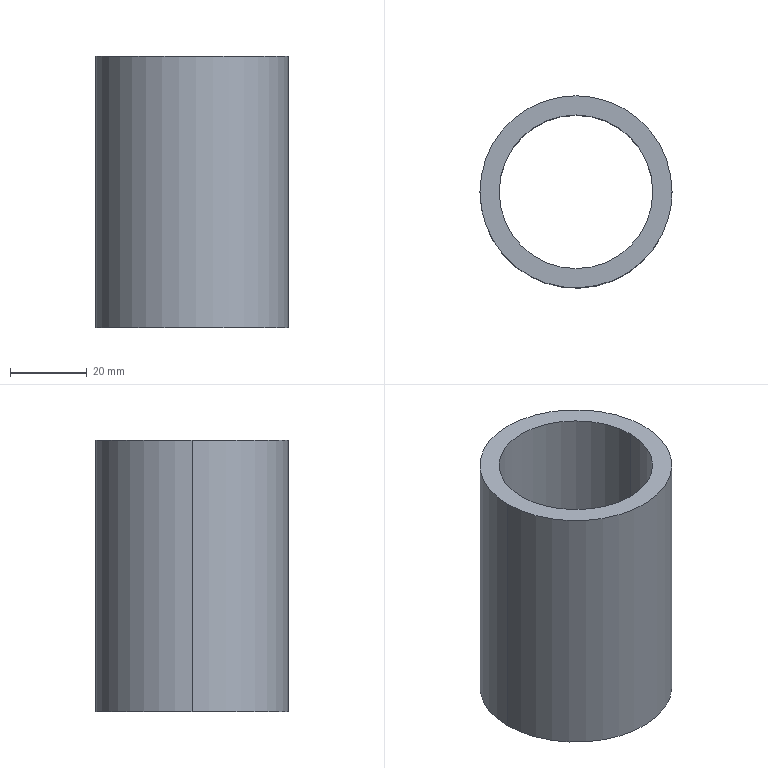Part | CATIA | 1 solid | 6 faces | box 50 x 50 x 70.6 mm | volume 49904 mm3 | cylinder 4 | plane 2 | commonest cylinder face diameters 40 x2 50 x2
STEP:
#1=CARTESIAN_POINT('',(35.,500.,-0.000000001));
#2=VERTEX_POINT('',#1);
#3=CARTESIAN_POINT('',(35.,500.,70.6));
#4=VERTEX_POINT('',#3);
#5=CARTESIAN_POINT('',(35.,500.,35.3));
#6=DIRECTION('',(0.,0.,1.));
#7=VECTOR('',#6,1.);
#8=LINE('',#5,#7);
#9=EDGE_CURVE('',#2,#4,#8,.T.);
#10=ORIENTED_EDGE('',*,*,#9,.F.);
#11=CARTESIAN_POINT('',(-15.,500.,-0.000000001));
#12=VERTEX_POINT('',#11);
#13=CARTESIAN_POINT('',(10.,500.,-0.000000001));
#14=DIRECTION('',(0.,0.,1.));
#15=AXIS2_PLACEMENT_3D('',#13,#14,$);
#16=CIRCLE('',#15,25.);
#17=EDGE_CURVE('',#2,#12,#16,.T.);
#18=ORIENTED_EDGE('',*,*,#17,.T.);
#19=CARTESIAN_POINT('',(-15.,500.,70.6));
#20=VERTEX_POINT('',#19);
#21=CARTESIAN_POINT('',(-15.,500.,35.3));
#22=DIRECTION('',(0.,0.,1.));
#23=VECTOR('',#22,1.);
#24=LINE('',#21,#23);
#25=EDGE_CURVE('',#12,#20,#24,.T.);
#26=ORIENTED_EDGE('',*,*,#25,.T.);
#27=CARTESIAN_POINT('',(10.,500.,70.6));
#28=DIRECTION('',(0.,0.,1.));
#29=AXIS2_PLACEMENT_3D('',#27,#28,$);
#30=CIRCLE('',#29,25.);
#31=EDGE_CURVE('',#4,#20,#30,.T.);
#32=ORIENTED_EDGE('',*,*,#31,.F.);
#33=EDGE_LOOP('',(#10,#18,#26,#32));
#34=FACE_OUTER_BOUND('',#33,.T.);
#35=CARTESIAN_POINT('',(10.,500.,35.3));
#36=DIRECTION('',(0.,0.,1.));
#37=DIRECTION('',(1.,0.,0.));
#38=AXIS2_PLACEMENT_3D('',#35,#36,#37);
#39=CYLINDRICAL_SURFACE('',#38,25.);
#40=ADVANCED_FACE('',(#34),#39,.T.);
#41=ORIENTED_EDGE('',*,*,#25,.F.);
#42=CARTESIAN_POINT('',(-15.,500.,0.));
#43=CARTESIAN_POINT('',(-15.,496.073,0.));
#44=CARTESIAN_POINT('',(-14.229,492.146,0.));
#45=CARTESIAN_POINT('',(-12.686,488.421,0.));
#46=CARTESIAN_POINT('',(-8.223,481.777,0.));
#47=CARTESIAN_POINT('',(-1.579,477.314,0.));
#48=CARTESIAN_POINT('',(2.146,475.771,0.));
#49=CARTESIAN_POINT('',(10.,474.229,0.));
#50=CARTESIAN_POINT('',(17.854,475.771,0.));
#51=CARTESIAN_POINT('',(21.579,477.314,0.));
#52=CARTESIAN_POINT('',(28.223,481.777,-0.000000001));
#53=CARTESIAN_POINT('',(32.686,488.421,-0.000000001));
#54=CARTESIAN_POINT('',(34.229,492.146,-0.000000001));
#55=CARTESIAN_POINT('',(35.,496.073,-0.000000001));
#56=CARTESIAN_POINT('',(35.,500.,-0.000000001));
#57=B_SPLINE_CURVE_WITH_KNOTS('',5,(#42,#43,#44,#45,#46,#47,#48,#49,#50,#51,#52,#53,#54,#55,#56),.UNSPECIFIED.,.F.,.U.,(6,3,3,3,6),(-39.27,-19.635,0.,19.635,39.27),.UNSPECIFIED.);
#58=EDGE_CURVE('',#12,#2,#57,.T.);
#59=ORIENTED_EDGE('',*,*,#58,.T.);
#60=ORIENTED_EDGE('',*,*,#9,.T.);
#61=CARTESIAN_POINT('',(-15.,500.,70.6));
#62=CARTESIAN_POINT('',(-15.,496.073,70.6));
#63=CARTESIAN_POINT('',(-14.229,492.146,70.6));
#64=CARTESIAN_POINT('',(-12.686,488.421,70.6));
#65=CARTESIAN_POINT('',(-8.223,481.777,70.6));
#66=CARTESIAN_POINT('',(-1.579,477.314,70.6));
#67=CARTESIAN_POINT('',(2.146,475.771,70.6));
#68=CARTESIAN_POINT('',(10.,474.229,70.6));
#69=CARTESIAN_POINT('',(17.854,475.771,70.6));
#70=CARTESIAN_POINT('',(21.579,477.314,70.6));
#71=CARTESIAN_POINT('',(28.223,481.777,70.6));
#72=CARTESIAN_POINT('',(32.686,488.421,70.6));
#73=CARTESIAN_POINT('',(34.229,492.146,70.6));
#74=CARTESIAN_POINT('',(35.,496.073,70.6));
#75=CARTESIAN_POINT('',(35.,500.,70.6));
#76=B_SPLINE_CURVE_WITH_KNOTS('',5,(#61,#62,#63,#64,#65,#66,#67,#68,#69,#70,#71,#72,#73,#74,#75),.UNSPECIFIED.,.F.,.U.,(6,3,3,3,6),(-39.27,-19.635,0.,19.635,39.27),.UNSPECIFIED.);
#77=EDGE_CURVE('',#20,#4,#76,.T.);
#78=ORIENTED_EDGE('',*,*,#77,.F.);
#79=EDGE_LOOP('',(#41,#59,#60,#78));
#80=FACE_OUTER_BOUND('',#79,.T.);
#81=CARTESIAN_POINT('',(10.,500.,35.3));
#82=DIRECTION('',(0.,0.,1.));
#83=DIRECTION('',(-1.,0.,0.));
#84=AXIS2_PLACEMENT_3D('',#81,#82,#83);
#85=CYLINDRICAL_SURFACE('',#84,25.);
#86=ADVANCED_FACE('',(#80),#85,.T.);
#87=ORIENTED_EDGE('',*,*,#58,.F.);
#88=ORIENTED_EDGE('',*,*,#17,.F.);
#89=EDGE_LOOP('',(#87,#88));
#90=FACE_OUTER_BOUND('',#89,.T.);
#91=CARTESIAN_POINT('',(30.,500.,0.));
#92=VERTEX_POINT('',#91);
#93=CARTESIAN_POINT('',(-10.,500.,-0.000000001));
#94=VERTEX_POINT('',#93);
#95=CARTESIAN_POINT('',(10.,500.,0.));
#96=DIRECTION('',(0.,0.,1.));
#97=AXIS2_PLACEMENT_3D('',#95,#96,$);
#98=CIRCLE('',#97,20.);
#99=EDGE_CURVE('',#92,#94,#98,.T.);
#100=ORIENTED_EDGE('',*,*,#99,.T.);
#101=CARTESIAN_POINT('',(10.,500.,0.));
#102=DIRECTION('',(0.,0.,1.));
#103=AXIS2_PLACEMENT_3D('',#101,#102,$);
#104=CIRCLE('',#103,20.);
#105=EDGE_CURVE('',#94,#92,#104,.T.);
#106=ORIENTED_EDGE('',*,*,#105,.T.);
#107=EDGE_LOOP('',(#100,#106));
#108=FACE_BOUND('',#107,.T.);
#109=CARTESIAN_POINT('',(0.,0.,0.));
#110=DIRECTION('',(0.,0.,1.));
#111=DIRECTION('',(1.,0.,0.));
#112=AXIS2_PLACEMENT_3D('',#109,#110,#111);
#113=PLANE('',#112);
#114=ADVANCED_FACE('',(#90,#108),#113,.F.);
#115=ORIENTED_EDGE('',*,*,#31,.T.);
#116=ORIENTED_EDGE('',*,*,#77,.T.);
#117=EDGE_LOOP('',(#115,#116));
#118=FACE_OUTER_BOUND('',#117,.T.);
#119=CARTESIAN_POINT('',(-10.,500.,70.6));
#120=VERTEX_POINT('',#119);
#121=CARTESIAN_POINT('',(30.,500.,70.6));
#122=VERTEX_POINT('',#121);
#123=CARTESIAN_POINT('',(10.,500.,70.6));
#124=DIRECTION('',(0.,0.,1.));
#125=AXIS2_PLACEMENT_3D('',#123,#124,$);
#126=CIRCLE('',#125,20.);
#127=EDGE_CURVE('',#120,#122,#126,.T.);
#128=ORIENTED_EDGE('',*,*,#127,.F.);
#129=CARTESIAN_POINT('',(10.,500.,70.6));
#130=DIRECTION('',(0.,0.,1.));
#131=AXIS2_PLACEMENT_3D('',#129,#130,$);
#132=CIRCLE('',#131,20.);
#133=EDGE_CURVE('',#122,#120,#132,.T.);
#134=ORIENTED_EDGE('',*,*,#133,.F.);
#135=EDGE_LOOP('',(#128,#134));
#136=FACE_BOUND('',#135,.T.);
#137=CARTESIAN_POINT('',(0.,0.,70.6));
#138=DIRECTION('',(0.,0.,1.));
#139=DIRECTION('',(1.,0.,0.));
#140=AXIS2_PLACEMENT_3D('',#137,#138,#139);
#141=PLANE('',#140);
#142=ADVANCED_FACE('',(#118,#136),#141,.T.);
#143=ORIENTED_EDGE('',*,*,#133,.T.);
#144=CARTESIAN_POINT('',(-10.,500.,35.3));
#145=DIRECTION('',(0.,0.,1.));
#146=VECTOR('',#145,1.);
#147=LINE('',#144,#146);
#148=EDGE_CURVE('',#94,#120,#147,.T.);
#149=ORIENTED_EDGE('',*,*,#148,.F.);
#150=ORIENTED_EDGE('',*,*,#99,.F.);
#151=CARTESIAN_POINT('',(30.,500.,35.3));
#152=DIRECTION('',(0.,0.,1.));
#153=VECTOR('',#152,1.);
#154=LINE('',#151,#153);
#155=EDGE_CURVE('',#92,#122,#154,.T.);
#156=ORIENTED_EDGE('',*,*,#155,.T.);
#157=EDGE_LOOP('',(#143,#149,#150,#156));
#158=FACE_OUTER_BOUND('',#157,.T.);
#159=CARTESIAN_POINT('',(10.,500.,35.3));
#160=DIRECTION('',(0.,0.,1.));
#161=DIRECTION('',(1.,0.,0.));
#162=AXIS2_PLACEMENT_3D('',#159,#160,#161);
#163=CYLINDRICAL_SURFACE('',#162,20.);
#164=ADVANCED_FACE('',(#158),#163,.F.);
#165=ORIENTED_EDGE('',*,*,#127,.T.);
#166=ORIENTED_EDGE('',*,*,#155,.F.);
#167=ORIENTED_EDGE('',*,*,#105,.F.);
#168=ORIENTED_EDGE('',*,*,#148,.T.);
#169=EDGE_LOOP('',(#165,#166,#167,#168));
#170=FACE_OUTER_BOUND('',#169,.T.);
#171=CARTESIAN_POINT('',(10.,500.,35.3));
#172=DIRECTION('',(0.,0.,1.));
#173=DIRECTION('',(-1.,0.,0.));
#174=AXIS2_PLACEMENT_3D('',#171,#172,#173);
#175=CYLINDRICAL_SURFACE('',#174,20.);
#176=ADVANCED_FACE('',(#170),#175,.F.);
#177=CLOSED_SHELL('',(#40,#86,#114,#142,#164,#176));
#178=MANIFOLD_SOLID_BREP('',#177);
#179=(LENGTH_UNIT()NAMED_UNIT(*)SI_UNIT(.MILLI.,.METRE.));
#180=UNCERTAINTY_MEASURE_WITH_UNIT(LENGTH_MEASURE(0.005),#179,'','');
#181=(NAMED_UNIT(*)PLANE_ANGLE_UNIT()SI_UNIT($,.RADIAN.));
#182=(NAMED_UNIT(*)SI_UNIT($,.STERADIAN.)SOLID_ANGLE_UNIT());
#183=(GEOMETRIC_REPRESENTATION_CONTEXT(3)GLOBAL_UNCERTAINTY_ASSIGNED_CONTEXT((#180))GLOBAL_UNIT_ASSIGNED_CONTEXT((#179,#181,#182))REPRESENTATION_CONTEXT('',''));
#184=ADVANCED_BREP_SHAPE_REPRESENTATION('',(#178),#183);